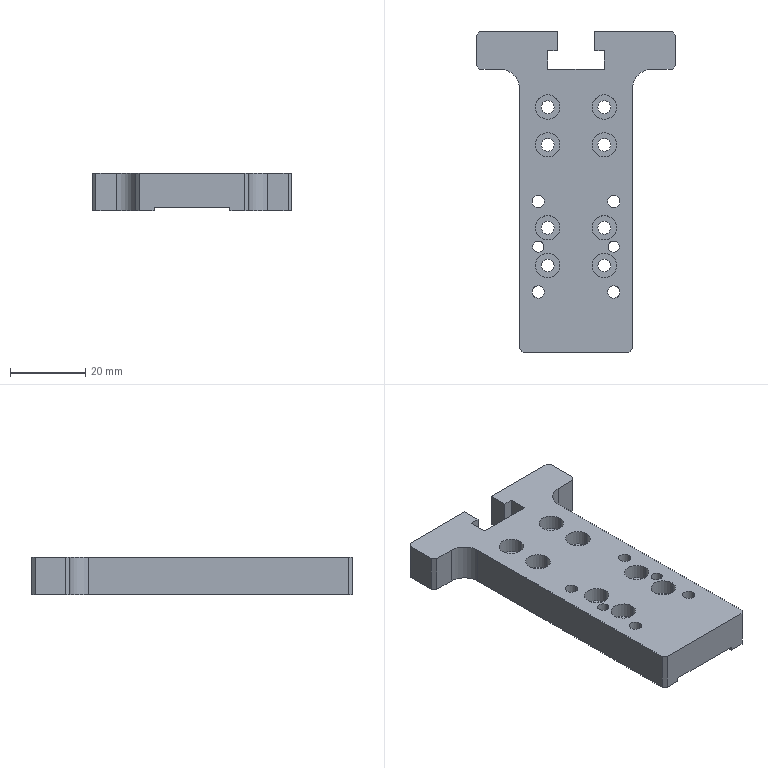Part | STEP file | PN_0071 Mount electronic clip s longitudinal manipulator slide rail plate | 1 solid | 88 faces | box 53 x 85 x 10 mm | volume 23160 mm3 | cylinder 46 | plane 42 | commonest cylinder face diameters 3.4 x16 6.5 x16 3.3 x8 3 x4 10 x2